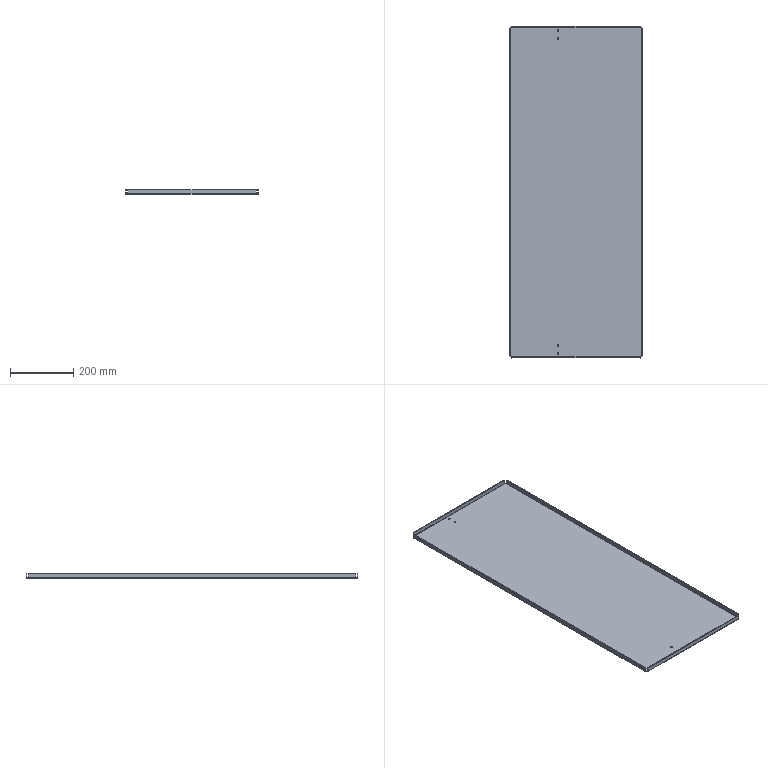Part | SolidWorks | features BaseBody 1 | 1 solid | 58 faces | box 418 x 1046 x 15 mm | volume 1176215 mm3 | plane 42 | cylinder 16 | commonest cylinder face diameters 5.5 x8 1.473 x4 6.473 x4